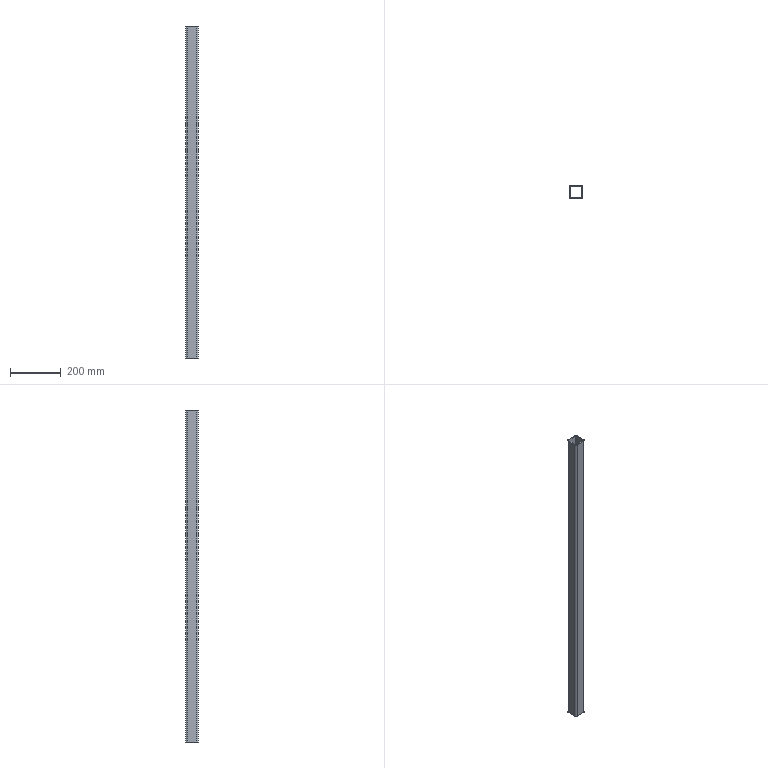Part | SolidWorks | 1 solid | 18 faces | box 50 x 50 x 1305 mm | volume 705774 mm3 | plane 10 | cylinder 8 | commonest cylinder face diameters 6 x4 12 x4
STEP:
#1=CARTESIAN_POINT('',(19.,25.,652.5));
#2=VERTEX_POINT('',#1);
#3=CARTESIAN_POINT('',(25.,19.,652.5));
#4=VERTEX_POINT('',#3);
#5=CARTESIAN_POINT('',(19.,19.,652.5));
#6=DIRECTION('',(0.,0.,-1.));
#7=DIRECTION('',(-1.,0.,0.));
#8=AXIS2_PLACEMENT_3D('',#5,#6,#7);
#9=CIRCLE('',#8,6.);
#10=EDGE_CURVE('',#2,#4,#9,.T.);
#11=ORIENTED_EDGE('',*,*,#10,.T.);
#12=CARTESIAN_POINT('',(25.,19.,-652.5));
#13=VERTEX_POINT('',#12);
#14=CARTESIAN_POINT('',(25.,19.,-652.5));
#15=DIRECTION('',(0.,0.,1.));
#16=VECTOR('',#15,1000.);
#17=LINE('',#14,#16);
#18=EDGE_CURVE('',#13,#4,#17,.T.);
#19=ORIENTED_EDGE('',*,*,#18,.F.);
#20=CARTESIAN_POINT('',(19.,25.,-652.5));
#21=VERTEX_POINT('',#20);
#22=CARTESIAN_POINT('',(19.,19.,-652.5));
#23=DIRECTION('',(0.,0.,-1.));
#24=DIRECTION('',(-1.,0.,0.));
#25=AXIS2_PLACEMENT_3D('',#22,#23,#24);
#26=CIRCLE('',#25,6.);
#27=EDGE_CURVE('',#21,#13,#26,.T.);
#28=ORIENTED_EDGE('',*,*,#27,.F.);
#29=CARTESIAN_POINT('',(19.,25.,-652.5));
#30=DIRECTION('',(0.,0.,1.));
#31=VECTOR('',#30,1000.);
#32=LINE('',#29,#31);
#33=EDGE_CURVE('',#21,#2,#32,.T.);
#34=ORIENTED_EDGE('',*,*,#33,.T.);
#35=EDGE_LOOP('',(#11,#19,#28,#34));
#36=FACE_OUTER_BOUND('',#35,.T.);
#37=CARTESIAN_POINT('',(19.,19.,-652.5));
#38=DIRECTION('',(0.,0.,1.));
#39=DIRECTION('',(1.,0.,0.));
#40=AXIS2_PLACEMENT_3D('',#37,#38,#39);
#41=CYLINDRICAL_SURFACE('',#40,6.);
#42=ADVANCED_FACE('',(#36),#41,.T.);
#43=CARTESIAN_POINT('',(25.,-19.,652.5));
#44=VERTEX_POINT('',#43);
#45=CARTESIAN_POINT('',(25.,19.,652.5));
#46=DIRECTION('',(0.,-1.,0.));
#47=VECTOR('',#46,1000.);
#48=LINE('',#45,#47);
#49=EDGE_CURVE('',#4,#44,#48,.T.);
#50=ORIENTED_EDGE('',*,*,#49,.T.);
#51=CARTESIAN_POINT('',(25.,-19.,-652.5));
#52=VERTEX_POINT('',#51);
#53=CARTESIAN_POINT('',(25.,-19.,-652.5));
#54=DIRECTION('',(0.,0.,1.));
#55=VECTOR('',#54,1000.);
#56=LINE('',#53,#55);
#57=EDGE_CURVE('',#52,#44,#56,.T.);
#58=ORIENTED_EDGE('',*,*,#57,.F.);
#59=CARTESIAN_POINT('',(25.,19.,-652.5));
#60=DIRECTION('',(0.,-1.,0.));
#61=VECTOR('',#60,1000.);
#62=LINE('',#59,#61);
#63=EDGE_CURVE('',#13,#52,#62,.T.);
#64=ORIENTED_EDGE('',*,*,#63,.F.);
#65=ORIENTED_EDGE('',*,*,#18,.T.);
#66=EDGE_LOOP('',(#50,#58,#64,#65));
#67=FACE_OUTER_BOUND('',#66,.T.);
#68=CARTESIAN_POINT('',(25.,19.,-652.5));
#69=DIRECTION('',(-1.,0.,0.));
#70=DIRECTION('',(0.,0.,1.));
#71=AXIS2_PLACEMENT_3D('',#68,#69,#70);
#72=PLANE('',#71);
#73=ADVANCED_FACE('',(#67),#72,.F.);
#74=CARTESIAN_POINT('',(19.,-25.,652.5));
#75=VERTEX_POINT('',#74);
#76=CARTESIAN_POINT('',(19.,-19.,652.5));
#77=DIRECTION('',(0.,0.,-1.));
#78=DIRECTION('',(-1.,0.,0.));
#79=AXIS2_PLACEMENT_3D('',#76,#77,#78);
#80=CIRCLE('',#79,6.);
#81=EDGE_CURVE('',#44,#75,#80,.T.);
#82=ORIENTED_EDGE('',*,*,#81,.T.);
#83=CARTESIAN_POINT('',(19.,-25.,-652.5));
#84=VERTEX_POINT('',#83);
#85=CARTESIAN_POINT('',(19.,-25.,-652.5));
#86=DIRECTION('',(0.,0.,1.));
#87=VECTOR('',#86,1000.);
#88=LINE('',#85,#87);
#89=EDGE_CURVE('',#84,#75,#88,.T.);
#90=ORIENTED_EDGE('',*,*,#89,.F.);
#91=CARTESIAN_POINT('',(19.,-19.,-652.5));
#92=DIRECTION('',(0.,0.,-1.));
#93=DIRECTION('',(-1.,0.,0.));
#94=AXIS2_PLACEMENT_3D('',#91,#92,#93);
#95=CIRCLE('',#94,6.);
#96=EDGE_CURVE('',#52,#84,#95,.T.);
#97=ORIENTED_EDGE('',*,*,#96,.F.);
#98=ORIENTED_EDGE('',*,*,#57,.T.);
#99=EDGE_LOOP('',(#82,#90,#97,#98));
#100=FACE_OUTER_BOUND('',#99,.T.);
#101=CARTESIAN_POINT('',(19.,-19.,-652.5));
#102=DIRECTION('',(0.,0.,1.));
#103=DIRECTION('',(1.,0.,0.));
#104=AXIS2_PLACEMENT_3D('',#101,#102,#103);
#105=CYLINDRICAL_SURFACE('',#104,6.);
#106=ADVANCED_FACE('',(#100),#105,.T.);
#107=CARTESIAN_POINT('',(-19.,-25.,652.5));
#108=VERTEX_POINT('',#107);
#109=CARTESIAN_POINT('',(-19.,-25.,652.5));
#110=DIRECTION('',(-1.,0.,0.));
#111=VECTOR('',#110,1000.);
#112=LINE('',#109,#111);
#113=EDGE_CURVE('',#75,#108,#112,.T.);
#114=ORIENTED_EDGE('',*,*,#113,.T.);
#115=CARTESIAN_POINT('',(-19.,-25.,-652.5));
#116=VERTEX_POINT('',#115);
#117=CARTESIAN_POINT('',(-19.,-25.,-652.5));
#118=DIRECTION('',(0.,0.,1.));
#119=VECTOR('',#118,1000.);
#120=LINE('',#117,#119);
#121=EDGE_CURVE('',#116,#108,#120,.T.);
#122=ORIENTED_EDGE('',*,*,#121,.F.);
#123=CARTESIAN_POINT('',(-19.,-25.,-652.5));
#124=DIRECTION('',(-1.,0.,0.));
#125=VECTOR('',#124,1000.);
#126=LINE('',#123,#125);
#127=EDGE_CURVE('',#84,#116,#126,.T.);
#128=ORIENTED_EDGE('',*,*,#127,.F.);
#129=ORIENTED_EDGE('',*,*,#89,.T.);
#130=EDGE_LOOP('',(#114,#122,#128,#129));
#131=FACE_OUTER_BOUND('',#130,.T.);
#132=CARTESIAN_POINT('',(-19.,-25.,-652.5));
#133=DIRECTION('',(0.,1.,0.));
#134=DIRECTION('',(0.,0.,1.));
#135=AXIS2_PLACEMENT_3D('',#132,#133,#134);
#136=PLANE('',#135);
#137=ADVANCED_FACE('',(#131),#136,.F.);
#138=CARTESIAN_POINT('',(-25.,-19.,652.5));
#139=VERTEX_POINT('',#138);
#140=CARTESIAN_POINT('',(-19.,-19.,652.5));
#141=DIRECTION('',(0.,0.,-1.));
#142=DIRECTION('',(-1.,0.,0.));
#143=AXIS2_PLACEMENT_3D('',#140,#141,#142);
#144=CIRCLE('',#143,6.);
#145=EDGE_CURVE('',#108,#139,#144,.T.);
#146=ORIENTED_EDGE('',*,*,#145,.T.);
#147=CARTESIAN_POINT('',(-25.,-19.,-652.5));
#148=VERTEX_POINT('',#147);
#149=CARTESIAN_POINT('',(-25.,-19.,-652.5));
#150=DIRECTION('',(0.,0.,1.));
#151=VECTOR('',#150,1000.);
#152=LINE('',#149,#151);
#153=EDGE_CURVE('',#148,#139,#152,.T.);
#154=ORIENTED_EDGE('',*,*,#153,.F.);
#155=CARTESIAN_POINT('',(-19.,-19.,-652.5));
#156=DIRECTION('',(0.,0.,-1.));
#157=DIRECTION('',(-1.,0.,0.));
#158=AXIS2_PLACEMENT_3D('',#155,#156,#157);
#159=CIRCLE('',#158,6.);
#160=EDGE_CURVE('',#116,#148,#159,.T.);
#161=ORIENTED_EDGE('',*,*,#160,.F.);
#162=ORIENTED_EDGE('',*,*,#121,.T.);
#163=EDGE_LOOP('',(#146,#154,#161,#162));
#164=FACE_OUTER_BOUND('',#163,.T.);
#165=CARTESIAN_POINT('',(-19.,-19.,-652.5));
#166=DIRECTION('',(0.,0.,1.));
#167=DIRECTION('',(1.,0.,0.));
#168=AXIS2_PLACEMENT_3D('',#165,#166,#167);
#169=CYLINDRICAL_SURFACE('',#168,6.);
#170=ADVANCED_FACE('',(#164),#169,.T.);
#171=CARTESIAN_POINT('',(-25.,19.,652.5));
#172=VERTEX_POINT('',#171);
#173=CARTESIAN_POINT('',(-25.,-19.,652.5));
#174=DIRECTION('',(0.,1.,0.));
#175=VECTOR('',#174,1000.);
#176=LINE('',#173,#175);
#177=EDGE_CURVE('',#139,#172,#176,.T.);
#178=ORIENTED_EDGE('',*,*,#177,.T.);
#179=CARTESIAN_POINT('',(-25.,19.,-652.5));
#180=VERTEX_POINT('',#179);
#181=CARTESIAN_POINT('',(-25.,19.,-652.5));
#182=DIRECTION('',(0.,0.,1.));
#183=VECTOR('',#182,1000.);
#184=LINE('',#181,#183);
#185=EDGE_CURVE('',#180,#172,#184,.T.);
#186=ORIENTED_EDGE('',*,*,#185,.F.);
#187=CARTESIAN_POINT('',(-25.,-19.,-652.5));
#188=DIRECTION('',(0.,1.,0.));
#189=VECTOR('',#188,1000.);
#190=LINE('',#187,#189);
#191=EDGE_CURVE('',#148,#180,#190,.T.);
#192=ORIENTED_EDGE('',*,*,#191,.F.);
#193=ORIENTED_EDGE('',*,*,#153,.T.);
#194=EDGE_LOOP('',(#178,#186,#192,#193));
#195=FACE_OUTER_BOUND('',#194,.T.);
#196=CARTESIAN_POINT('',(-25.,-19.,-652.5));
#197=DIRECTION('',(1.,0.,0.));
#198=DIRECTION('',(0.,0.,-1.));
#199=AXIS2_PLACEMENT_3D('',#196,#197,#198);
#200=PLANE('',#199);
#201=ADVANCED_FACE('',(#195),#200,.F.);
#202=CARTESIAN_POINT('',(-19.,25.,652.5));
#203=VERTEX_POINT('',#202);
#204=CARTESIAN_POINT('',(-19.,19.,652.5));
#205=DIRECTION('',(0.,0.,-1.));
#206=DIRECTION('',(-1.,0.,0.));
#207=AXIS2_PLACEMENT_3D('',#204,#205,#206);
#208=CIRCLE('',#207,6.);
#209=EDGE_CURVE('',#172,#203,#208,.T.);
#210=ORIENTED_EDGE('',*,*,#209,.T.);
#211=CARTESIAN_POINT('',(-19.,25.,-652.5));
#212=VERTEX_POINT('',#211);
#213=CARTESIAN_POINT('',(-19.,25.,-652.5));
#214=DIRECTION('',(0.,0.,1.));
#215=VECTOR('',#214,1000.);
#216=LINE('',#213,#215);
#217=EDGE_CURVE('',#212,#203,#216,.T.);
#218=ORIENTED_EDGE('',*,*,#217,.F.);
#219=CARTESIAN_POINT('',(-19.,19.,-652.5));
#220=DIRECTION('',(0.,0.,-1.));
#221=DIRECTION('',(-1.,0.,0.));
#222=AXIS2_PLACEMENT_3D('',#219,#220,#221);
#223=CIRCLE('',#222,6.);
#224=EDGE_CURVE('',#180,#212,#223,.T.);
#225=ORIENTED_EDGE('',*,*,#224,.F.);
#226=ORIENTED_EDGE('',*,*,#185,.T.);
#227=EDGE_LOOP('',(#210,#218,#225,#226));
#228=FACE_OUTER_BOUND('',#227,.T.);
#229=CARTESIAN_POINT('',(-19.,19.,-652.5));
#230=DIRECTION('',(0.,0.,1.));
#231=DIRECTION('',(1.,0.,0.));
#232=AXIS2_PLACEMENT_3D('',#229,#230,#231);
#233=CYLINDRICAL_SURFACE('',#232,6.);
#234=ADVANCED_FACE('',(#228),#233,.T.);
#235=CARTESIAN_POINT('',(22.,-19.,652.5));
#236=VERTEX_POINT('',#235);
#237=CARTESIAN_POINT('',(19.,-22.,652.5));
#238=VERTEX_POINT('',#237);
#239=CARTESIAN_POINT('',(19.,-19.,652.5));
#240=DIRECTION('',(0.,0.,-1.));
#241=DIRECTION('',(-1.,0.,0.));
#242=AXIS2_PLACEMENT_3D('',#239,#240,#241);
#243=CIRCLE('',#242,3.);
#244=EDGE_CURVE('',#236,#238,#243,.T.);
#245=ORIENTED_EDGE('',*,*,#244,.F.);
#246=CARTESIAN_POINT('',(22.,-19.,-652.5));
#247=VERTEX_POINT('',#246);
#248=CARTESIAN_POINT('',(22.,-19.,-652.5));
#249=DIRECTION('',(0.,0.,1.));
#250=VECTOR('',#249,1000.);
#251=LINE('',#248,#250);
#252=EDGE_CURVE('',#247,#236,#251,.T.);
#253=ORIENTED_EDGE('',*,*,#252,.F.);
#254=CARTESIAN_POINT('',(19.,-22.,-652.5));
#255=VERTEX_POINT('',#254);
#256=CARTESIAN_POINT('',(19.,-19.,-652.5));
#257=DIRECTION('',(0.,0.,-1.));
#258=DIRECTION('',(-1.,0.,0.));
#259=AXIS2_PLACEMENT_3D('',#256,#257,#258);
#260=CIRCLE('',#259,3.);
#261=EDGE_CURVE('',#247,#255,#260,.T.);
#262=ORIENTED_EDGE('',*,*,#261,.T.);
#263=CARTESIAN_POINT('',(19.,-22.,-652.5));
#264=DIRECTION('',(0.,0.,1.));
#265=VECTOR('',#264,1000.);
#266=LINE('',#263,#265);
#267=EDGE_CURVE('',#255,#238,#266,.T.);
#268=ORIENTED_EDGE('',*,*,#267,.T.);
#269=EDGE_LOOP('',(#245,#253,#262,#268));
#270=FACE_OUTER_BOUND('',#269,.T.);
#271=CARTESIAN_POINT('',(19.,-19.,-652.5));
#272=DIRECTION('',(0.,0.,1.));
#273=DIRECTION('',(1.,0.,0.));
#274=AXIS2_PLACEMENT_3D('',#271,#272,#273);
#275=CYLINDRICAL_SURFACE('',#274,3.);
#276=ADVANCED_FACE('',(#270),#275,.F.);
#277=CARTESIAN_POINT('',(22.,19.,652.5));
#278=VERTEX_POINT('',#277);
#279=CARTESIAN_POINT('',(22.,19.,652.5));
#280=DIRECTION('',(0.,-1.,0.));
#281=VECTOR('',#280,1000.);
#282=LINE('',#279,#281);
#283=EDGE_CURVE('',#278,#236,#282,.T.);
#284=ORIENTED_EDGE('',*,*,#283,.F.);
#285=CARTESIAN_POINT('',(22.,19.,-652.5));
#286=VERTEX_POINT('',#285);
#287=CARTESIAN_POINT('',(22.,19.,-652.5));
#288=DIRECTION('',(0.,0.,1.));
#289=VECTOR('',#288,1000.);
#290=LINE('',#287,#289);
#291=EDGE_CURVE('',#286,#278,#290,.T.);
#292=ORIENTED_EDGE('',*,*,#291,.F.);
#293=CARTESIAN_POINT('',(22.,19.,-652.5));
#294=DIRECTION('',(0.,-1.,0.));
#295=VECTOR('',#294,1000.);
#296=LINE('',#293,#295);
#297=EDGE_CURVE('',#286,#247,#296,.T.);
#298=ORIENTED_EDGE('',*,*,#297,.T.);
#299=ORIENTED_EDGE('',*,*,#252,.T.);
#300=EDGE_LOOP('',(#284,#292,#298,#299));
#301=FACE_OUTER_BOUND('',#300,.T.);
#302=CARTESIAN_POINT('',(22.,19.,-652.5));
#303=DIRECTION('',(-1.,0.,0.));
#304=DIRECTION('',(0.,0.,1.));
#305=AXIS2_PLACEMENT_3D('',#302,#303,#304);
#306=PLANE('',#305);
#307=ADVANCED_FACE('',(#301),#306,.T.);
#308=CARTESIAN_POINT('',(19.,22.,652.5));
#309=VERTEX_POINT('',#308);
#310=CARTESIAN_POINT('',(19.,19.,652.5));
#311=DIRECTION('',(0.,0.,-1.));
#312=DIRECTION('',(-1.,0.,0.));
#313=AXIS2_PLACEMENT_3D('',#310,#311,#312);
#314=CIRCLE('',#313,3.);
#315=EDGE_CURVE('',#309,#278,#314,.T.);
#316=ORIENTED_EDGE('',*,*,#315,.F.);
#317=CARTESIAN_POINT('',(19.,22.,-652.5));
#318=VERTEX_POINT('',#317);
#319=CARTESIAN_POINT('',(19.,22.,-652.5));
#320=DIRECTION('',(0.,0.,1.));
#321=VECTOR('',#320,1000.);
#322=LINE('',#319,#321);
#323=EDGE_CURVE('',#318,#309,#322,.T.);
#324=ORIENTED_EDGE('',*,*,#323,.F.);
#325=CARTESIAN_POINT('',(19.,19.,-652.5));
#326=DIRECTION('',(0.,0.,-1.));
#327=DIRECTION('',(-1.,0.,0.));
#328=AXIS2_PLACEMENT_3D('',#325,#326,#327);
#329=CIRCLE('',#328,3.);
#330=EDGE_CURVE('',#318,#286,#329,.T.);
#331=ORIENTED_EDGE('',*,*,#330,.T.);
#332=ORIENTED_EDGE('',*,*,#291,.T.);
#333=EDGE_LOOP('',(#316,#324,#331,#332));
#334=FACE_OUTER_BOUND('',#333,.T.);
#335=CARTESIAN_POINT('',(19.,19.,-652.5));
#336=DIRECTION('',(0.,0.,1.));
#337=DIRECTION('',(1.,0.,0.));
#338=AXIS2_PLACEMENT_3D('',#335,#336,#337);
#339=CYLINDRICAL_SURFACE('',#338,3.);
#340=ADVANCED_FACE('',(#334),#339,.F.);
#341=CARTESIAN_POINT('',(-19.,22.,652.5));
#342=VERTEX_POINT('',#341);
#343=CARTESIAN_POINT('',(19.,22.,652.5));
#344=DIRECTION('',(1.,0.,0.));
#345=VECTOR('',#344,1000.);
#346=LINE('',#343,#345);
#347=EDGE_CURVE('',#342,#309,#346,.T.);
#348=ORIENTED_EDGE('',*,*,#347,.F.);
#349=CARTESIAN_POINT('',(-19.,22.,-652.5));
#350=VERTEX_POINT('',#349);
#351=CARTESIAN_POINT('',(-19.,22.,-652.5));
#352=DIRECTION('',(0.,0.,1.));
#353=VECTOR('',#352,1000.);
#354=LINE('',#351,#353);
#355=EDGE_CURVE('',#350,#342,#354,.T.);
#356=ORIENTED_EDGE('',*,*,#355,.F.);
#357=CARTESIAN_POINT('',(19.,22.,-652.5));
#358=DIRECTION('',(1.,0.,0.));
#359=VECTOR('',#358,1000.);
#360=LINE('',#357,#359);
#361=EDGE_CURVE('',#350,#318,#360,.T.);
#362=ORIENTED_EDGE('',*,*,#361,.T.);
#363=ORIENTED_EDGE('',*,*,#323,.T.);
#364=EDGE_LOOP('',(#348,#356,#362,#363));
#365=FACE_OUTER_BOUND('',#364,.T.);
#366=CARTESIAN_POINT('',(19.,22.,-652.5));
#367=DIRECTION('',(0.,-1.,0.));
#368=DIRECTION('',(0.,0.,-1.));
#369=AXIS2_PLACEMENT_3D('',#366,#367,#368);
#370=PLANE('',#369);
#371=ADVANCED_FACE('',(#365),#370,.T.);
#372=CARTESIAN_POINT('',(-22.,19.,652.5));
#373=VERTEX_POINT('',#372);
#374=CARTESIAN_POINT('',(-19.,19.,652.5));
#375=DIRECTION('',(0.,0.,-1.));
#376=DIRECTION('',(-1.,0.,0.));
#377=AXIS2_PLACEMENT_3D('',#374,#375,#376);
#378=CIRCLE('',#377,3.);
#379=EDGE_CURVE('',#373,#342,#378,.T.);
#380=ORIENTED_EDGE('',*,*,#379,.F.);
#381=CARTESIAN_POINT('',(-22.,19.,-652.5));
#382=VERTEX_POINT('',#381);
#383=CARTESIAN_POINT('',(-22.,19.,-652.5));
#384=DIRECTION('',(0.,0.,1.));
#385=VECTOR('',#384,1000.);
#386=LINE('',#383,#385);
#387=EDGE_CURVE('',#382,#373,#386,.T.);
#388=ORIENTED_EDGE('',*,*,#387,.F.);
#389=CARTESIAN_POINT('',(-19.,19.,-652.5));
#390=DIRECTION('',(0.,0.,-1.));
#391=DIRECTION('',(-1.,0.,0.));
#392=AXIS2_PLACEMENT_3D('',#389,#390,#391);
#393=CIRCLE('',#392,3.);
#394=EDGE_CURVE('',#382,#350,#393,.T.);
#395=ORIENTED_EDGE('',*,*,#394,.T.);
#396=ORIENTED_EDGE('',*,*,#355,.T.);
#397=EDGE_LOOP('',(#380,#388,#395,#396));
#398=FACE_OUTER_BOUND('',#397,.T.);
#399=CARTESIAN_POINT('',(-19.,19.,-652.5));
#400=DIRECTION('',(0.,0.,1.));
#401=DIRECTION('',(1.,0.,0.));
#402=AXIS2_PLACEMENT_3D('',#399,#400,#401);
#403=CYLINDRICAL_SURFACE('',#402,3.);
#404=ADVANCED_FACE('',(#398),#403,.F.);
#405=CARTESIAN_POINT('',(-22.,-19.,652.5));
#406=VERTEX_POINT('',#405);
#407=CARTESIAN_POINT('',(-22.,-19.,652.5));
#408=DIRECTION('',(0.,1.,0.));
#409=VECTOR('',#408,1000.);
#410=LINE('',#407,#409);
#411=EDGE_CURVE('',#406,#373,#410,.T.);
#412=ORIENTED_EDGE('',*,*,#411,.F.);
#413=CARTESIAN_POINT('',(-22.,-19.,-652.5));
#414=VERTEX_POINT('',#413);
#415=CARTESIAN_POINT('',(-22.,-19.,-652.5));
#416=DIRECTION('',(0.,0.,1.));
#417=VECTOR('',#416,1000.);
#418=LINE('',#415,#417);
#419=EDGE_CURVE('',#414,#406,#418,.T.);
#420=ORIENTED_EDGE('',*,*,#419,.F.);
#421=CARTESIAN_POINT('',(-22.,-19.,-652.5));
#422=DIRECTION('',(0.,1.,0.));
#423=VECTOR('',#422,1000.);
#424=LINE('',#421,#423);
#425=EDGE_CURVE('',#414,#382,#424,.T.);
#426=ORIENTED_EDGE('',*,*,#425,.T.);
#427=ORIENTED_EDGE('',*,*,#387,.T.);
#428=EDGE_LOOP('',(#412,#420,#426,#427));
#429=FACE_OUTER_BOUND('',#428,.T.);
#430=CARTESIAN_POINT('',(-22.,-19.,-652.5));
#431=DIRECTION('',(1.,0.,0.));
#432=DIRECTION('',(0.,0.,-1.));
#433=AXIS2_PLACEMENT_3D('',#430,#431,#432);
#434=PLANE('',#433);
#435=ADVANCED_FACE('',(#429),#434,.T.);
#436=CARTESIAN_POINT('',(-19.,-22.,652.5));
#437=VERTEX_POINT('',#436);
#438=CARTESIAN_POINT('',(-19.,-19.,652.5));
#439=DIRECTION('',(0.,0.,-1.));
#440=DIRECTION('',(-1.,0.,0.));
#441=AXIS2_PLACEMENT_3D('',#438,#439,#440);
#442=CIRCLE('',#441,3.);
#443=EDGE_CURVE('',#437,#406,#442,.T.);
#444=ORIENTED_EDGE('',*,*,#443,.F.);
#445=CARTESIAN_POINT('',(-19.,-22.,-652.5));
#446=VERTEX_POINT('',#445);
#447=CARTESIAN_POINT('',(-19.,-22.,-652.5));
#448=DIRECTION('',(0.,0.,1.));
#449=VECTOR('',#448,1000.);
#450=LINE('',#447,#449);
#451=EDGE_CURVE('',#446,#437,#450,.T.);
#452=ORIENTED_EDGE('',*,*,#451,.F.);
#453=CARTESIAN_POINT('',(-19.,-19.,-652.5));
#454=DIRECTION('',(0.,0.,-1.));
#455=DIRECTION('',(-1.,0.,0.));
#456=AXIS2_PLACEMENT_3D('',#453,#454,#455);
#457=CIRCLE('',#456,3.);
#458=EDGE_CURVE('',#446,#414,#457,.T.);
#459=ORIENTED_EDGE('',*,*,#458,.T.);
#460=ORIENTED_EDGE('',*,*,#419,.T.);
#461=EDGE_LOOP('',(#444,#452,#459,#460));
#462=FACE_OUTER_BOUND('',#461,.T.);
#463=CARTESIAN_POINT('',(-19.,-19.,-652.5));
#464=DIRECTION('',(0.,0.,1.));
#465=DIRECTION('',(1.,0.,0.));
#466=AXIS2_PLACEMENT_3D('',#463,#464,#465);
#467=CYLINDRICAL_SURFACE('',#466,3.);
#468=ADVANCED_FACE('',(#462),#467,.F.);
#469=CARTESIAN_POINT('',(-19.,-22.,652.5));
#470=DIRECTION('',(-1.,0.,0.));
#471=VECTOR('',#470,1000.);
#472=LINE('',#469,#471);
#473=EDGE_CURVE('',#238,#437,#472,.T.);
#474=ORIENTED_EDGE('',*,*,#473,.F.);
#475=ORIENTED_EDGE('',*,*,#267,.F.);
#476=CARTESIAN_POINT('',(-19.,-22.,-652.5));
#477=DIRECTION('',(-1.,0.,0.));
#478=VECTOR('',#477,1000.);
#479=LINE('',#476,#478);
#480=EDGE_CURVE('',#255,#446,#479,.T.);
#481=ORIENTED_EDGE('',*,*,#480,.T.);
#482=ORIENTED_EDGE('',*,*,#451,.T.);
#483=EDGE_LOOP('',(#474,#475,#481,#482));
#484=FACE_OUTER_BOUND('',#483,.T.);
#485=CARTESIAN_POINT('',(-19.,-22.,-652.5));
#486=DIRECTION('',(0.,1.,0.));
#487=DIRECTION('',(0.,0.,1.));
#488=AXIS2_PLACEMENT_3D('',#485,#486,#487);
#489=PLANE('',#488);
#490=ADVANCED_FACE('',(#484),#489,.T.);
#491=CARTESIAN_POINT('',(19.,25.,652.5));
#492=DIRECTION('',(1.,0.,0.));
#493=VECTOR('',#492,1000.);
#494=LINE('',#491,#493);
#495=EDGE_CURVE('',#203,#2,#494,.T.);
#496=ORIENTED_EDGE('',*,*,#495,.T.);
#497=ORIENTED_EDGE('',*,*,#33,.F.);
#498=CARTESIAN_POINT('',(19.,25.,-652.5));
#499=DIRECTION('',(1.,0.,0.));
#500=VECTOR('',#499,1000.);
#501=LINE('',#498,#500);
#502=EDGE_CURVE('',#212,#21,#501,.T.);
#503=ORIENTED_EDGE('',*,*,#502,.F.);
#504=ORIENTED_EDGE('',*,*,#217,.T.);
#505=EDGE_LOOP('',(#496,#497,#503,#504));
#506=FACE_OUTER_BOUND('',#505,.T.);
#507=CARTESIAN_POINT('',(19.,25.,-652.5));
#508=DIRECTION('',(0.,-1.,0.));
#509=DIRECTION('',(0.,0.,-1.));
#510=AXIS2_PLACEMENT_3D('',#507,#508,#509);
#511=PLANE('',#510);
#512=ADVANCED_FACE('',(#506),#511,.F.);
#513=ORIENTED_EDGE('',*,*,#261,.F.);
#514=ORIENTED_EDGE('',*,*,#297,.F.);
#515=ORIENTED_EDGE('',*,*,#330,.F.);
#516=ORIENTED_EDGE('',*,*,#361,.F.);
#517=ORIENTED_EDGE('',*,*,#394,.F.);
#518=ORIENTED_EDGE('',*,*,#425,.F.);
#519=ORIENTED_EDGE('',*,*,#458,.F.);
#520=ORIENTED_EDGE('',*,*,#480,.F.);
#521=EDGE_LOOP('',(#513,#514,#515,#516,#517,#518,#519,#520));
#522=FACE_BOUND('',#521,.T.);
#523=ORIENTED_EDGE('',*,*,#27,.T.);
#524=ORIENTED_EDGE('',*,*,#63,.T.);
#525=ORIENTED_EDGE('',*,*,#96,.T.);
#526=ORIENTED_EDGE('',*,*,#127,.T.);
#527=ORIENTED_EDGE('',*,*,#160,.T.);
#528=ORIENTED_EDGE('',*,*,#191,.T.);
#529=ORIENTED_EDGE('',*,*,#224,.T.);
#530=ORIENTED_EDGE('',*,*,#502,.T.);
#531=EDGE_LOOP('',(#523,#524,#525,#526,#527,#528,#529,#530));
#532=FACE_OUTER_BOUND('',#531,.T.);
#533=CARTESIAN_POINT('',(19.,19.,-652.5));
#534=DIRECTION('',(0.,0.,-1.));
#535=DIRECTION('',(-1.,0.,0.));
#536=AXIS2_PLACEMENT_3D('',#533,#534,#535);
#537=PLANE('',#536);
#538=ADVANCED_FACE('',(#522,#532),#537,.T.);
#539=ORIENTED_EDGE('',*,*,#244,.T.);
#540=ORIENTED_EDGE('',*,*,#473,.T.);
#541=ORIENTED_EDGE('',*,*,#443,.T.);
#542=ORIENTED_EDGE('',*,*,#411,.T.);
#543=ORIENTED_EDGE('',*,*,#379,.T.);
#544=ORIENTED_EDGE('',*,*,#347,.T.);
#545=ORIENTED_EDGE('',*,*,#315,.T.);
#546=ORIENTED_EDGE('',*,*,#283,.T.);
#547=EDGE_LOOP('',(#539,#540,#541,#542,#543,#544,#545,#546));
#548=FACE_BOUND('',#547,.T.);
#549=ORIENTED_EDGE('',*,*,#10,.F.);
#550=ORIENTED_EDGE('',*,*,#495,.F.);
#551=ORIENTED_EDGE('',*,*,#209,.F.);
#552=ORIENTED_EDGE('',*,*,#177,.F.);
#553=ORIENTED_EDGE('',*,*,#145,.F.);
#554=ORIENTED_EDGE('',*,*,#113,.F.);
#555=ORIENTED_EDGE('',*,*,#81,.F.);
#556=ORIENTED_EDGE('',*,*,#49,.F.);
#557=EDGE_LOOP('',(#549,#550,#551,#552,#553,#554,#555,#556));
#558=FACE_OUTER_BOUND('',#557,.T.);
#559=CARTESIAN_POINT('',(19.,19.,652.5));
#560=DIRECTION('',(0.,0.,-1.));
#561=DIRECTION('',(-1.,0.,0.));
#562=AXIS2_PLACEMENT_3D('',#559,#560,#561);
#563=PLANE('',#562);
#564=ADVANCED_FACE('',(#548,#558),#563,.F.);
#565=CLOSED_SHELL('',(#42,#73,#106,#137,#170,#201,#234,#276,#307,#340,#371,#404,#435,#468,#490,#512,#538,#564));
#566=MANIFOLD_SOLID_BREP('',#565);
#567=CARTESIAN_POINT('',(0.,0.,0.));
#568=DIRECTION('',(0.,0.,1.));
#569=DIRECTION('',(1.,0.,0.));
#570=AXIS2_PLACEMENT_3D('',#567,#568,#569);
#571=(LENGTH_UNIT()NAMED_UNIT(*)SI_UNIT(.MILLI.,.METRE.));
#572=UNCERTAINTY_MEASURE_WITH_UNIT(LENGTH_MEASURE(0.00001),#571,'','');
#573=(NAMED_UNIT(*)PLANE_ANGLE_UNIT()SI_UNIT($,.RADIAN.));
#574=(NAMED_UNIT(*)SI_UNIT($,.STERADIAN.)SOLID_ANGLE_UNIT());
#575=(GEOMETRIC_REPRESENTATION_CONTEXT(3)GLOBAL_UNCERTAINTY_ASSIGNED_CONTEXT((#572))GLOBAL_UNIT_ASSIGNED_CONTEXT((#571,#573,#574))REPRESENTATION_CONTEXT('',''));
#576=ADVANCED_BREP_SHAPE_REPRESENTATION('',(#566,#570),#575);